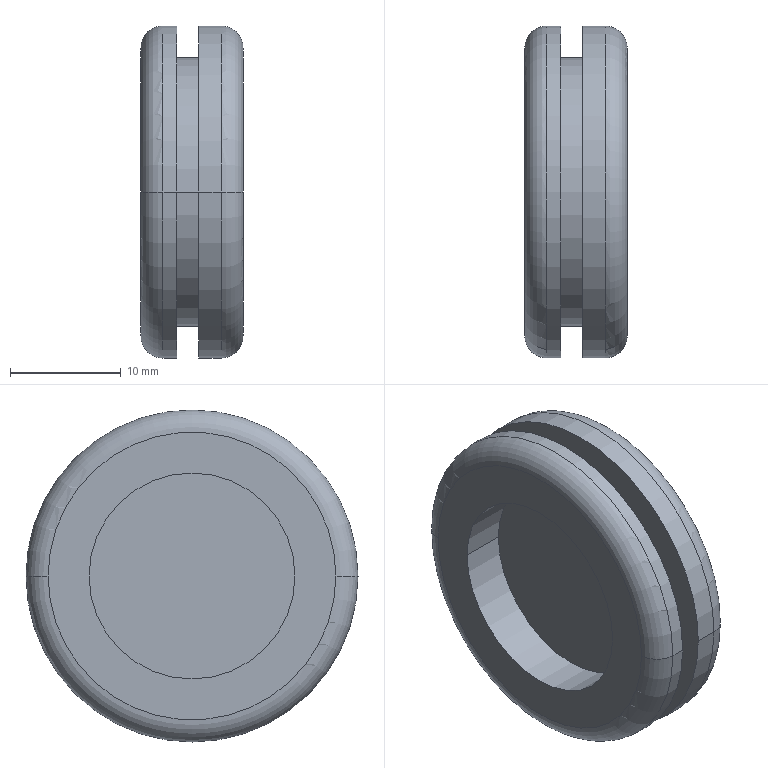Part | STEP file | 60008141 | 1 solid | 20 faces | box 9.25 x 30 x 30 mm | volume 3450 mm3 | cylinder 10 | plane 6 | torus 4 | commonest cylinder face diameters 18.6 x4 30 x4 24.3 x2
STEP:
#1=CARTESIAN_POINT('',(0.,0.,0.));
#2=DIRECTION('',(0.,0.,1.));
#3=DIRECTION('',(1.,0.,0.));
#4=AXIS2_PLACEMENT_3D('',#1,#2,#3);
#5=CARTESIAN_POINT('',(-4.25,9.3,0.));
#6=VERTEX_POINT('',#5);
#7=CARTESIAN_POINT('',(-0.25,9.3,0.));
#8=VERTEX_POINT('',#7);
#9=CARTESIAN_POINT('',(-4.25,9.3,0.));
#10=DIRECTION('',(1.,0.,0.));
#11=VECTOR('',#10,1.);
#12=LINE('',#9,#11);
#13=CARTESIAN_POINT('',(-4.463,0.,0.));
#14=DIRECTION('',(1.,0.,0.));
#15=DIRECTION('',(0.,-1.,0.));
#16=AXIS2_PLACEMENT_3D('',#13,#14,#15);
#17=CYLINDRICAL_SURFACE('',#16,9.3);
#18=CARTESIAN_POINT('',(3.142,0.2125));
#19=DIRECTION('',(0.,1.));
#20=VECTOR('',#19,1.);
#21=LINE('',#18,#20);
#22=(GEOMETRIC_REPRESENTATION_CONTEXT(2)PARAMETRIC_REPRESENTATION_CONTEXT()REPRESENTATION_CONTEXT('',''));
#23=DEFINITIONAL_REPRESENTATION('',(#21),#22);
#24=PCURVE('',#17,#23);
#25=CARTESIAN_POINT('',(-4.463,0.,0.));
#26=DIRECTION('',(1.,0.,0.));
#27=DIRECTION('',(0.,-1.,0.));
#28=AXIS2_PLACEMENT_3D('',#25,#26,#27);
#29=CYLINDRICAL_SURFACE('',#28,9.3);
#30=CARTESIAN_POINT('',(3.142,0.2125));
#31=DIRECTION('',(0.,1.));
#32=VECTOR('',#31,1.);
#33=LINE('',#30,#32);
#34=(GEOMETRIC_REPRESENTATION_CONTEXT(2)PARAMETRIC_REPRESENTATION_CONTEXT()REPRESENTATION_CONTEXT('',''));
#35=DEFINITIONAL_REPRESENTATION('',(#33),#34);
#36=PCURVE('',#29,#35);
#37=SURFACE_CURVE('',#12,(#24,#36),.PCURVE_S1.);
#38=EDGE_CURVE('',#6,#8,#37,.T.);
#39=ORIENTED_EDGE('',*,*,#38,.F.);
#40=CARTESIAN_POINT('',(-4.25,-9.3,0.));
#41=VERTEX_POINT('',#40);
#42=CARTESIAN_POINT('',(-4.25,0.,0.));
#43=DIRECTION('',(1.,0.,0.));
#44=DIRECTION('',(0.,1.,0.));
#45=AXIS2_PLACEMENT_3D('',#42,#43,#44);
#46=CIRCLE('',#45,9.3);
#47=CARTESIAN_POINT('',(3.142,0.2125));
#48=DIRECTION('',(1.,0.));
#49=VECTOR('',#48,1.);
#50=LINE('',#47,#49);
#51=(GEOMETRIC_REPRESENTATION_CONTEXT(2)PARAMETRIC_REPRESENTATION_CONTEXT()REPRESENTATION_CONTEXT('',''));
#52=DEFINITIONAL_REPRESENTATION('',(#50),#51);
#53=PCURVE('',#17,#52);
#54=CARTESIAN_POINT('',(-4.25,0.,0.));
#55=DIRECTION('',(1.,0.,0.));
#56=DIRECTION('',(0.,-1.,0.));
#57=AXIS2_PLACEMENT_3D('',#54,#55,#56);
#58=PLANE('',#57);
#59=CARTESIAN_POINT('',(0.,0.));
#60=DIRECTION('',(-1.,0.));
#61=AXIS2_PLACEMENT_2D('',#59,#60);
#62=CIRCLE('',#61,9.3);
#63=(GEOMETRIC_REPRESENTATION_CONTEXT(2)PARAMETRIC_REPRESENTATION_CONTEXT()REPRESENTATION_CONTEXT('',''));
#64=DEFINITIONAL_REPRESENTATION('',(#62),#63);
#65=PCURVE('',#58,#64);
#66=SURFACE_CURVE('',#46,(#53,#65),.PCURVE_S1.);
#67=EDGE_CURVE('',#6,#41,#66,.T.);
#68=ORIENTED_EDGE('',*,*,#67,.T.);
#69=CARTESIAN_POINT('',(-0.25,-9.3,0.));
#70=VERTEX_POINT('',#69);
#71=CARTESIAN_POINT('',(-4.25,-9.3,0.));
#72=DIRECTION('',(1.,0.,0.));
#73=VECTOR('',#72,1.);
#74=LINE('',#71,#73);
#75=CARTESIAN_POINT('',(6.283,0.2125));
#76=DIRECTION('',(0.,1.));
#77=VECTOR('',#76,1.);
#78=LINE('',#75,#77);
#79=(GEOMETRIC_REPRESENTATION_CONTEXT(2)PARAMETRIC_REPRESENTATION_CONTEXT()REPRESENTATION_CONTEXT('',''));
#80=DEFINITIONAL_REPRESENTATION('',(#78),#79);
#81=PCURVE('',#17,#80);
#82=CARTESIAN_POINT('',(0.,0.2125));
#83=DIRECTION('',(0.,1.));
#84=VECTOR('',#83,1.);
#85=LINE('',#82,#84);
#86=(GEOMETRIC_REPRESENTATION_CONTEXT(2)PARAMETRIC_REPRESENTATION_CONTEXT()REPRESENTATION_CONTEXT('',''));
#87=DEFINITIONAL_REPRESENTATION('',(#85),#86);
#88=PCURVE('',#29,#87);
#89=SURFACE_CURVE('',#74,(#81,#88),.PCURVE_S1.);
#90=EDGE_CURVE('',#41,#70,#89,.T.);
#91=ORIENTED_EDGE('',*,*,#90,.T.);
#92=CARTESIAN_POINT('',(-0.25,0.,0.));
#93=DIRECTION('',(1.,0.,0.));
#94=DIRECTION('',(0.,1.,0.));
#95=AXIS2_PLACEMENT_3D('',#92,#93,#94);
#96=CIRCLE('',#95,9.3);
#97=CARTESIAN_POINT('',(3.142,4.213));
#98=DIRECTION('',(1.,0.));
#99=VECTOR('',#98,1.);
#100=LINE('',#97,#99);
#101=(GEOMETRIC_REPRESENTATION_CONTEXT(2)PARAMETRIC_REPRESENTATION_CONTEXT()REPRESENTATION_CONTEXT('',''));
#102=DEFINITIONAL_REPRESENTATION('',(#100),#101);
#103=PCURVE('',#17,#102);
#104=CARTESIAN_POINT('',(-0.25,0.,0.));
#105=DIRECTION('',(1.,0.,0.));
#106=DIRECTION('',(0.,-1.,0.));
#107=AXIS2_PLACEMENT_3D('',#104,#105,#106);
#108=PLANE('',#107);
#109=CARTESIAN_POINT('',(0.,0.));
#110=DIRECTION('',(-1.,0.));
#111=AXIS2_PLACEMENT_2D('',#109,#110);
#112=CIRCLE('',#111,9.3);
#113=(GEOMETRIC_REPRESENTATION_CONTEXT(2)PARAMETRIC_REPRESENTATION_CONTEXT()REPRESENTATION_CONTEXT('',''));
#114=DEFINITIONAL_REPRESENTATION('',(#112),#113);
#115=PCURVE('',#108,#114);
#116=SURFACE_CURVE('',#96,(#103,#115),.PCURVE_S1.);
#117=EDGE_CURVE('',#8,#70,#116,.T.);
#118=ORIENTED_EDGE('',*,*,#117,.F.);
#119=EDGE_LOOP('',(#39,#68,#91,#118));
#120=FACE_BOUND('',#119,.F.);
#121=ADVANCED_FACE('',(#120),#17,.F.);
#122=ORIENTED_EDGE('',*,*,#38,.T.);
#123=CARTESIAN_POINT('',(-0.25,0.,0.));
#124=DIRECTION('',(-1.,0.,0.));
#125=DIRECTION('',(0.,1.,0.));
#126=AXIS2_PLACEMENT_3D('',#123,#124,#125);
#127=CIRCLE('',#126,9.3);
#128=CARTESIAN_POINT('',(3.142,4.213));
#129=DIRECTION('',(-1.,0.));
#130=VECTOR('',#129,1.);
#131=LINE('',#128,#130);
#132=(GEOMETRIC_REPRESENTATION_CONTEXT(2)PARAMETRIC_REPRESENTATION_CONTEXT()REPRESENTATION_CONTEXT('',''));
#133=DEFINITIONAL_REPRESENTATION('',(#131),#132);
#134=PCURVE('',#29,#133);
#135=CARTESIAN_POINT('',(-9.3,0.));
#136=CARTESIAN_POINT('',(-9.3,16.108));
#137=CARTESIAN_POINT('',(4.65,8.054));
#138=CARTESIAN_POINT('',(18.6,0.));
#139=CARTESIAN_POINT('',(4.65,-8.054));
#140=CARTESIAN_POINT('',(-9.3,-16.108));
#141=CARTESIAN_POINT('',(-9.3,0.));
#142=(BOUNDED_CURVE()B_SPLINE_CURVE(2,(#135,#136,#137,#138,#139,#140,#141),.UNSPECIFIED.,.T.,.F.)B_SPLINE_CURVE_WITH_KNOTS((1,2,2,2,2,1),(-2.094,0.,2.094,4.189,6.283,8.378),.UNSPECIFIED.)CURVE()GEOMETRIC_REPRESENTATION_ITEM()RATIONAL_B_SPLINE_CURVE((1.,0.5,1.,0.5,1.,0.5,1.))REPRESENTATION_ITEM(''));
#143=(GEOMETRIC_REPRESENTATION_CONTEXT(2)PARAMETRIC_REPRESENTATION_CONTEXT()REPRESENTATION_CONTEXT('',''));
#144=DEFINITIONAL_REPRESENTATION('',(#142),#143);
#145=PCURVE('',#108,#144);
#146=SURFACE_CURVE('',#127,(#134,#145),.PCURVE_S1.);
#147=EDGE_CURVE('',#8,#70,#146,.T.);
#148=ORIENTED_EDGE('',*,*,#147,.T.);
#149=ORIENTED_EDGE('',*,*,#90,.F.);
#150=CARTESIAN_POINT('',(-4.25,0.,0.));
#151=DIRECTION('',(-1.,0.,0.));
#152=DIRECTION('',(0.,1.,0.));
#153=AXIS2_PLACEMENT_3D('',#150,#151,#152);
#154=CIRCLE('',#153,9.3);
#155=CARTESIAN_POINT('',(3.142,0.2125));
#156=DIRECTION('',(-1.,0.));
#157=VECTOR('',#156,1.);
#158=LINE('',#155,#157);
#159=(GEOMETRIC_REPRESENTATION_CONTEXT(2)PARAMETRIC_REPRESENTATION_CONTEXT()REPRESENTATION_CONTEXT('',''));
#160=DEFINITIONAL_REPRESENTATION('',(#158),#159);
#161=PCURVE('',#29,#160);
#162=CARTESIAN_POINT('',(-9.3,0.));
#163=CARTESIAN_POINT('',(-9.3,16.108));
#164=CARTESIAN_POINT('',(4.65,8.054));
#165=CARTESIAN_POINT('',(18.6,0.));
#166=CARTESIAN_POINT('',(4.65,-8.054));
#167=CARTESIAN_POINT('',(-9.3,-16.108));
#168=CARTESIAN_POINT('',(-9.3,0.));
#169=(BOUNDED_CURVE()B_SPLINE_CURVE(2,(#162,#163,#164,#165,#166,#167,#168),.UNSPECIFIED.,.T.,.F.)B_SPLINE_CURVE_WITH_KNOTS((1,2,2,2,2,1),(-2.094,0.,2.094,4.189,6.283,8.378),.UNSPECIFIED.)CURVE()GEOMETRIC_REPRESENTATION_ITEM()RATIONAL_B_SPLINE_CURVE((1.,0.5,1.,0.5,1.,0.5,1.))REPRESENTATION_ITEM(''));
#170=(GEOMETRIC_REPRESENTATION_CONTEXT(2)PARAMETRIC_REPRESENTATION_CONTEXT()REPRESENTATION_CONTEXT('',''));
#171=DEFINITIONAL_REPRESENTATION('',(#169),#170);
#172=PCURVE('',#58,#171);
#173=SURFACE_CURVE('',#154,(#161,#172),.PCURVE_S1.);
#174=EDGE_CURVE('',#6,#41,#173,.T.);
#175=ORIENTED_EDGE('',*,*,#174,.F.);
#176=EDGE_LOOP('',(#122,#148,#149,#175));
#177=FACE_BOUND('',#176,.F.);
#178=ADVANCED_FACE('',(#177),#29,.F.);
#179=ORIENTED_EDGE('',*,*,#147,.F.);
#180=ORIENTED_EDGE('',*,*,#117,.T.);
#181=EDGE_LOOP('',(#179,#180));
#182=FACE_BOUND('',#181,.F.);
#183=ADVANCED_FACE('',(#182),#108,.F.);
#184=CARTESIAN_POINT('',(-4.25,13.,0.));
#185=VERTEX_POINT('',#184);
#186=CARTESIAN_POINT('',(-4.25,-13.,0.));
#187=VERTEX_POINT('',#186);
#188=CARTESIAN_POINT('',(-4.25,0.,0.));
#189=DIRECTION('',(1.,0.,0.));
#190=DIRECTION('',(0.,1.,0.));
#191=AXIS2_PLACEMENT_3D('',#188,#189,#190);
#192=CIRCLE('',#191,13.);
#193=CARTESIAN_POINT('',(0.,0.));
#194=DIRECTION('',(-1.,0.));
#195=AXIS2_PLACEMENT_2D('',#193,#194);
#196=CIRCLE('',#195,13.);
#197=(GEOMETRIC_REPRESENTATION_CONTEXT(2)PARAMETRIC_REPRESENTATION_CONTEXT()REPRESENTATION_CONTEXT('',''));
#198=DEFINITIONAL_REPRESENTATION('',(#196),#197);
#199=PCURVE('',#58,#198);
#200=CARTESIAN_POINT('',(-2.25,0.,0.));
#201=DIRECTION('',(1.,0.,0.));
#202=DIRECTION('',(0.,-1.,0.));
#203=AXIS2_PLACEMENT_3D('',#200,#201,#202);
#204=TOROIDAL_SURFACE('',#203,13.,2.);
#205=CARTESIAN_POINT('',(3.142,4.712));
#206=DIRECTION('',(1.,0.));
#207=VECTOR('',#206,1.);
#208=LINE('',#205,#207);
#209=(GEOMETRIC_REPRESENTATION_CONTEXT(2)PARAMETRIC_REPRESENTATION_CONTEXT()REPRESENTATION_CONTEXT('',''));
#210=DEFINITIONAL_REPRESENTATION('',(#208),#209);
#211=PCURVE('',#204,#210);
#212=SURFACE_CURVE('',#192,(#199,#211),.PCURVE_S1.);
#213=EDGE_CURVE('',#185,#187,#212,.T.);
#214=ORIENTED_EDGE('',*,*,#213,.T.);
#215=CARTESIAN_POINT('',(-4.25,0.,0.));
#216=DIRECTION('',(-1.,0.,0.));
#217=DIRECTION('',(0.,1.,0.));
#218=AXIS2_PLACEMENT_3D('',#215,#216,#217);
#219=CIRCLE('',#218,13.);
#220=CARTESIAN_POINT('',(-13.,0.));
#221=CARTESIAN_POINT('',(-13.,22.517));
#222=CARTESIAN_POINT('',(6.5,11.258));
#223=CARTESIAN_POINT('',(26.,0.));
#224=CARTESIAN_POINT('',(6.5,-11.258));
#225=CARTESIAN_POINT('',(-13.,-22.517));
#226=CARTESIAN_POINT('',(-13.,0.));
#227=(BOUNDED_CURVE()B_SPLINE_CURVE(2,(#220,#221,#222,#223,#224,#225,#226),.UNSPECIFIED.,.T.,.F.)B_SPLINE_CURVE_WITH_KNOTS((1,2,2,2,2,1),(-2.094,0.,2.094,4.189,6.283,8.378),.UNSPECIFIED.)CURVE()GEOMETRIC_REPRESENTATION_ITEM()RATIONAL_B_SPLINE_CURVE((1.,0.5,1.,0.5,1.,0.5,1.))REPRESENTATION_ITEM(''));
#228=(GEOMETRIC_REPRESENTATION_CONTEXT(2)PARAMETRIC_REPRESENTATION_CONTEXT()REPRESENTATION_CONTEXT('',''));
#229=DEFINITIONAL_REPRESENTATION('',(#227),#228);
#230=PCURVE('',#58,#229);
#231=CARTESIAN_POINT('',(-2.25,0.,0.));
#232=DIRECTION('',(1.,0.,0.));
#233=DIRECTION('',(0.,-1.,0.));
#234=AXIS2_PLACEMENT_3D('',#231,#232,#233);
#235=TOROIDAL_SURFACE('',#234,13.,2.);
#236=CARTESIAN_POINT('',(3.142,4.712));
#237=DIRECTION('',(-1.,0.));
#238=VECTOR('',#237,1.);
#239=LINE('',#236,#238);
#240=(GEOMETRIC_REPRESENTATION_CONTEXT(2)PARAMETRIC_REPRESENTATION_CONTEXT()REPRESENTATION_CONTEXT('',''));
#241=DEFINITIONAL_REPRESENTATION('',(#239),#240);
#242=PCURVE('',#235,#241);
#243=SURFACE_CURVE('',#219,(#230,#242),.PCURVE_S1.);
#244=EDGE_CURVE('',#185,#187,#243,.T.);
#245=ORIENTED_EDGE('',*,*,#244,.F.);
#246=EDGE_LOOP('',(#214,#245));
#247=FACE_BOUND('',#246,.F.);
#248=ORIENTED_EDGE('',*,*,#174,.T.);
#249=ORIENTED_EDGE('',*,*,#67,.F.);
#250=EDGE_LOOP('',(#248,#249));
#251=FACE_BOUND('',#250,.F.);
#252=ADVANCED_FACE('',(#247,#251),#58,.F.);
#253=ORIENTED_EDGE('',*,*,#213,.T.);
#254=CARTESIAN_POINT('',(-2.25,-15.,0.));
#255=VERTEX_POINT('',#254);
#256=CARTESIAN_POINT('',(-2.25,-13.,0.));
#257=DIRECTION('',(0.,0.,-1.));
#258=DIRECTION('',(0.,-1.,0.));
#259=AXIS2_PLACEMENT_3D('',#256,#257,#258);
#260=CIRCLE('',#259,2.);
#261=CARTESIAN_POINT('',(6.283,6.283));
#262=DIRECTION('',(0.,-1.));
#263=VECTOR('',#262,1.);
#264=LINE('',#261,#263);
#265=(GEOMETRIC_REPRESENTATION_CONTEXT(2)PARAMETRIC_REPRESENTATION_CONTEXT()REPRESENTATION_CONTEXT('',''));
#266=DEFINITIONAL_REPRESENTATION('',(#264),#265);
#267=PCURVE('',#204,#266);
#268=CARTESIAN_POINT('',(0.,6.283));
#269=DIRECTION('',(0.,-1.));
#270=VECTOR('',#269,1.);
#271=LINE('',#268,#270);
#272=(GEOMETRIC_REPRESENTATION_CONTEXT(2)PARAMETRIC_REPRESENTATION_CONTEXT()REPRESENTATION_CONTEXT('',''));
#273=DEFINITIONAL_REPRESENTATION('',(#271),#272);
#274=PCURVE('',#235,#273);
#275=SURFACE_CURVE('',#260,(#267,#274),.PCURVE_S1.);
#276=EDGE_CURVE('',#255,#187,#275,.T.);
#277=ORIENTED_EDGE('',*,*,#276,.F.);
#278=CARTESIAN_POINT('',(-2.25,15.,0.));
#279=VERTEX_POINT('',#278);
#280=CARTESIAN_POINT('',(-2.25,0.,0.));
#281=DIRECTION('',(1.,0.,0.));
#282=DIRECTION('',(0.,1.,0.));
#283=AXIS2_PLACEMENT_3D('',#280,#281,#282);
#284=CIRCLE('',#283,15.);
#285=CARTESIAN_POINT('',(3.142,6.283));
#286=DIRECTION('',(1.,0.));
#287=VECTOR('',#286,1.);
#288=LINE('',#285,#287);
#289=(GEOMETRIC_REPRESENTATION_CONTEXT(2)PARAMETRIC_REPRESENTATION_CONTEXT()REPRESENTATION_CONTEXT('',''));
#290=DEFINITIONAL_REPRESENTATION('',(#288),#289);
#291=PCURVE('',#204,#290);
#292=CARTESIAN_POINT('',(-4.463,0.,0.));
#293=DIRECTION('',(1.,0.,0.));
#294=DIRECTION('',(0.,-1.,0.));
#295=AXIS2_PLACEMENT_3D('',#292,#293,#294);
#296=CYLINDRICAL_SURFACE('',#295,15.);
#297=CARTESIAN_POINT('',(3.142,2.212));
#298=DIRECTION('',(1.,0.));
#299=VECTOR('',#298,1.);
#300=LINE('',#297,#299);
#301=(GEOMETRIC_REPRESENTATION_CONTEXT(2)PARAMETRIC_REPRESENTATION_CONTEXT()REPRESENTATION_CONTEXT('',''));
#302=DEFINITIONAL_REPRESENTATION('',(#300),#301);
#303=PCURVE('',#296,#302);
#304=SURFACE_CURVE('',#284,(#291,#303),.PCURVE_S1.);
#305=EDGE_CURVE('',#279,#255,#304,.T.);
#306=ORIENTED_EDGE('',*,*,#305,.F.);
#307=CARTESIAN_POINT('',(-2.25,13.,0.));
#308=DIRECTION('',(0.,0.,1.));
#309=DIRECTION('',(0.,1.,0.));
#310=AXIS2_PLACEMENT_3D('',#307,#308,#309);
#311=CIRCLE('',#310,2.);
#312=CARTESIAN_POINT('',(3.142,6.283));
#313=DIRECTION('',(0.,-1.));
#314=VECTOR('',#313,1.);
#315=LINE('',#312,#314);
#316=(GEOMETRIC_REPRESENTATION_CONTEXT(2)PARAMETRIC_REPRESENTATION_CONTEXT()REPRESENTATION_CONTEXT('',''));
#317=DEFINITIONAL_REPRESENTATION('',(#315),#316);
#318=PCURVE('',#204,#317);
#319=CARTESIAN_POINT('',(3.142,6.283));
#320=DIRECTION('',(0.,-1.));
#321=VECTOR('',#320,1.);
#322=LINE('',#319,#321);
#323=(GEOMETRIC_REPRESENTATION_CONTEXT(2)PARAMETRIC_REPRESENTATION_CONTEXT()REPRESENTATION_CONTEXT('',''));
#324=DEFINITIONAL_REPRESENTATION('',(#322),#323);
#325=PCURVE('',#235,#324);
#326=SURFACE_CURVE('',#311,(#318,#325),.PCURVE_S1.);
#327=EDGE_CURVE('',#279,#185,#326,.T.);
#328=ORIENTED_EDGE('',*,*,#327,.T.);
#329=EDGE_LOOP('',(#253,#277,#306,#328));
#330=FACE_BOUND('',#329,.T.);
#331=ADVANCED_FACE('',(#330),#204,.T.);
#332=CARTESIAN_POINT('',(-2.25,0.,0.));
#333=DIRECTION('',(-1.,0.,0.));
#334=DIRECTION('',(0.,1.,0.));
#335=AXIS2_PLACEMENT_3D('',#332,#333,#334);
#336=CIRCLE('',#335,15.);
#337=CARTESIAN_POINT('',(3.142,6.283));
#338=DIRECTION('',(-1.,0.));
#339=VECTOR('',#338,1.);
#340=LINE('',#337,#339);
#341=(GEOMETRIC_REPRESENTATION_CONTEXT(2)PARAMETRIC_REPRESENTATION_CONTEXT()REPRESENTATION_CONTEXT('',''));
#342=DEFINITIONAL_REPRESENTATION('',(#340),#341);
#343=PCURVE('',#235,#342);
#344=CARTESIAN_POINT('',(-4.463,0.,0.));
#345=DIRECTION('',(1.,0.,0.));
#346=DIRECTION('',(0.,-1.,0.));
#347=AXIS2_PLACEMENT_3D('',#344,#345,#346);
#348=CYLINDRICAL_SURFACE('',#347,15.);
#349=CARTESIAN_POINT('',(3.142,2.212));
#350=DIRECTION('',(-1.,0.));
#351=VECTOR('',#350,1.);
#352=LINE('',#349,#351);
#353=(GEOMETRIC_REPRESENTATION_CONTEXT(2)PARAMETRIC_REPRESENTATION_CONTEXT()REPRESENTATION_CONTEXT('',''));
#354=DEFINITIONAL_REPRESENTATION('',(#352),#353);
#355=PCURVE('',#348,#354);
#356=SURFACE_CURVE('',#336,(#343,#355),.PCURVE_S1.);
#357=EDGE_CURVE('',#279,#255,#356,.T.);
#358=ORIENTED_EDGE('',*,*,#357,.T.);
#359=ORIENTED_EDGE('',*,*,#276,.T.);
#360=ORIENTED_EDGE('',*,*,#244,.F.);
#361=ORIENTED_EDGE('',*,*,#327,.F.);
#362=EDGE_LOOP('',(#358,#359,#360,#361));
#363=FACE_BOUND('',#362,.T.);
#364=ADVANCED_FACE('',(#363),#235,.T.);
#365=CARTESIAN_POINT('',(-1.,15.,0.));
#366=VERTEX_POINT('',#365);
#367=CARTESIAN_POINT('',(-1.,-15.,0.));
#368=VERTEX_POINT('',#367);
#369=CARTESIAN_POINT('',(-1.,0.,0.));
#370=DIRECTION('',(-1.,0.,0.));
#371=DIRECTION('',(0.,1.,0.));
#372=AXIS2_PLACEMENT_3D('',#369,#370,#371);
#373=CIRCLE('',#372,15.);
#374=CARTESIAN_POINT('',(3.142,3.462));
#375=DIRECTION('',(-1.,0.));
#376=VECTOR('',#375,1.);
#377=LINE('',#374,#376);
#378=(GEOMETRIC_REPRESENTATION_CONTEXT(2)PARAMETRIC_REPRESENTATION_CONTEXT()REPRESENTATION_CONTEXT('',''));
#379=DEFINITIONAL_REPRESENTATION('',(#377),#378);
#380=PCURVE('',#348,#379);
#381=CARTESIAN_POINT('',(-1.,0.,0.));
#382=DIRECTION('',(1.,0.,0.));
#383=DIRECTION('',(0.,-1.,0.));
#384=AXIS2_PLACEMENT_3D('',#381,#382,#383);
#385=PLANE('',#384);
#386=CARTESIAN_POINT('',(-15.,0.));
#387=CARTESIAN_POINT('',(-15.,25.981));
#388=CARTESIAN_POINT('',(7.5,12.99));
#389=CARTESIAN_POINT('',(30.,0.));
#390=CARTESIAN_POINT('',(7.5,-12.99));
#391=CARTESIAN_POINT('',(-15.,-25.981));
#392=CARTESIAN_POINT('',(-15.,0.));
#393=(BOUNDED_CURVE()B_SPLINE_CURVE(2,(#386,#387,#388,#389,#390,#391,#392),.UNSPECIFIED.,.T.,.F.)B_SPLINE_CURVE_WITH_KNOTS((1,2,2,2,2,1),(-2.094,0.,2.094,4.189,6.283,8.378),.UNSPECIFIED.)CURVE()GEOMETRIC_REPRESENTATION_ITEM()RATIONAL_B_SPLINE_CURVE((1.,0.5,1.,0.5,1.,0.5,1.))REPRESENTATION_ITEM(''));
#394=(GEOMETRIC_REPRESENTATION_CONTEXT(2)PARAMETRIC_REPRESENTATION_CONTEXT()REPRESENTATION_CONTEXT('',''));
#395=DEFINITIONAL_REPRESENTATION('',(#393),#394);
#396=PCURVE('',#385,#395);
#397=SURFACE_CURVE('',#373,(#380,#396),.PCURVE_S1.);
#398=EDGE_CURVE('',#366,#368,#397,.T.);
#399=ORIENTED_EDGE('',*,*,#398,.T.);
#400=CARTESIAN_POINT('',(-1.,-15.,0.));
#401=DIRECTION('',(-1.,0.,0.));
#402=VECTOR('',#401,1.);
#403=LINE('',#400,#402);
#404=CARTESIAN_POINT('',(0.,3.462));
#405=DIRECTION('',(0.,-1.));
#406=VECTOR('',#405,1.);
#407=LINE('',#404,#406);
#408=(GEOMETRIC_REPRESENTATION_CONTEXT(2)PARAMETRIC_REPRESENTATION_CONTEXT()REPRESENTATION_CONTEXT('',''));
#409=DEFINITIONAL_REPRESENTATION('',(#407),#408);
#410=PCURVE('',#348,#409);
#411=CARTESIAN_POINT('',(6.283,3.462));
#412=DIRECTION('',(0.,-1.));
#413=VECTOR('',#412,1.);
#414=LINE('',#411,#413);
#415=(GEOMETRIC_REPRESENTATION_CONTEXT(2)PARAMETRIC_REPRESENTATION_CONTEXT()REPRESENTATION_CONTEXT('',''));
#416=DEFINITIONAL_REPRESENTATION('',(#414),#415);
#417=PCURVE('',#296,#416);
#418=SURFACE_CURVE('',#403,(#410,#417),.PCURVE_S1.);
#419=EDGE_CURVE('',#368,#255,#418,.T.);
#420=ORIENTED_EDGE('',*,*,#419,.T.);
#421=ORIENTED_EDGE('',*,*,#357,.F.);
#422=CARTESIAN_POINT('',(-1.,15.,0.));
#423=DIRECTION('',(-1.,0.,0.));
#424=VECTOR('',#423,1.);
#425=LINE('',#422,#424);
#426=CARTESIAN_POINT('',(3.142,3.462));
#427=DIRECTION('',(0.,-1.));
#428=VECTOR('',#427,1.);
#429=LINE('',#426,#428);
#430=(GEOMETRIC_REPRESENTATION_CONTEXT(2)PARAMETRIC_REPRESENTATION_CONTEXT()REPRESENTATION_CONTEXT('',''));
#431=DEFINITIONAL_REPRESENTATION('',(#429),#430);
#432=PCURVE('',#348,#431);
#433=CARTESIAN_POINT('',(3.142,3.462));
#434=DIRECTION('',(0.,-1.));
#435=VECTOR('',#434,1.);
#436=LINE('',#433,#435);
#437=(GEOMETRIC_REPRESENTATION_CONTEXT(2)PARAMETRIC_REPRESENTATION_CONTEXT()REPRESENTATION_CONTEXT('',''));
#438=DEFINITIONAL_REPRESENTATION('',(#436),#437);
#439=PCURVE('',#296,#438);
#440=SURFACE_CURVE('',#425,(#432,#439),.PCURVE_S1.);
#441=EDGE_CURVE('',#366,#279,#440,.T.);
#442=ORIENTED_EDGE('',*,*,#441,.F.);
#443=EDGE_LOOP('',(#399,#420,#421,#442));
#444=FACE_BOUND('',#443,.T.);
#445=ADVANCED_FACE('',(#444),#348,.T.);
#446=ORIENTED_EDGE('',*,*,#305,.T.);
#447=ORIENTED_EDGE('',*,*,#419,.F.);
#448=CARTESIAN_POINT('',(-1.,0.,0.));
#449=DIRECTION('',(1.,0.,0.));
#450=DIRECTION('',(0.,1.,0.));
#451=AXIS2_PLACEMENT_3D('',#448,#449,#450);
#452=CIRCLE('',#451,15.);
#453=CARTESIAN_POINT('',(3.142,3.462));
#454=DIRECTION('',(1.,0.));
#455=VECTOR('',#454,1.);
#456=LINE('',#453,#455);
#457=(GEOMETRIC_REPRESENTATION_CONTEXT(2)PARAMETRIC_REPRESENTATION_CONTEXT()REPRESENTATION_CONTEXT('',''));
#458=DEFINITIONAL_REPRESENTATION('',(#456),#457);
#459=PCURVE('',#296,#458);
#460=CARTESIAN_POINT('',(0.,0.));
#461=DIRECTION('',(-1.,0.));
#462=AXIS2_PLACEMENT_2D('',#460,#461);
#463=CIRCLE('',#462,15.);
#464=(GEOMETRIC_REPRESENTATION_CONTEXT(2)PARAMETRIC_REPRESENTATION_CONTEXT()REPRESENTATION_CONTEXT('',''));
#465=DEFINITIONAL_REPRESENTATION('',(#463),#464);
#466=PCURVE('',#385,#465);
#467=SURFACE_CURVE('',#452,(#459,#466),.PCURVE_S1.);
#468=EDGE_CURVE('',#366,#368,#467,.T.);
#469=ORIENTED_EDGE('',*,*,#468,.F.);
#470=ORIENTED_EDGE('',*,*,#441,.T.);
#471=EDGE_LOOP('',(#446,#447,#469,#470));
#472=FACE_BOUND('',#471,.T.);
#473=ADVANCED_FACE('',(#472),#296,.T.);
#474=ORIENTED_EDGE('',*,*,#398,.T.);
#475=ORIENTED_EDGE('',*,*,#468,.F.);
#476=EDGE_LOOP('',(#474,#475));
#477=FACE_BOUND('',#476,.F.);
#478=CARTESIAN_POINT('',(-1.,12.15,0.));
#479=VERTEX_POINT('',#478);
#480=CARTESIAN_POINT('',(-1.,-12.15,0.));
#481=VERTEX_POINT('',#480);
#482=CARTESIAN_POINT('',(-1.,0.,0.));
#483=DIRECTION('',(1.,0.,0.));
#484=DIRECTION('',(0.,1.,0.));
#485=AXIS2_PLACEMENT_3D('',#482,#483,#484);
#486=CIRCLE('',#485,12.15);
#487=CARTESIAN_POINT('',(0.,0.));
#488=DIRECTION('',(-1.,0.));
#489=AXIS2_PLACEMENT_2D('',#487,#488);
#490=CIRCLE('',#489,12.15);
#491=(GEOMETRIC_REPRESENTATION_CONTEXT(2)PARAMETRIC_REPRESENTATION_CONTEXT()REPRESENTATION_CONTEXT('',''));
#492=DEFINITIONAL_REPRESENTATION('',(#490),#491);
#493=PCURVE('',#385,#492);
#494=CARTESIAN_POINT('',(-4.463,0.,0.));
#495=DIRECTION('',(1.,0.,0.));
#496=DIRECTION('',(0.,-1.,0.));
#497=AXIS2_PLACEMENT_3D('',#494,#495,#496);
#498=CYLINDRICAL_SURFACE('',#497,12.15);
#499=CARTESIAN_POINT('',(3.142,3.462));
#500=DIRECTION('',(1.,0.));
#501=VECTOR('',#500,1.);
#502=LINE('',#499,#501);
#503=(GEOMETRIC_REPRESENTATION_CONTEXT(2)PARAMETRIC_REPRESENTATION_CONTEXT()REPRESENTATION_CONTEXT('',''));
#504=DEFINITIONAL_REPRESENTATION('',(#502),#503);
#505=PCURVE('',#498,#504);
#506=SURFACE_CURVE('',#486,(#493,#505),.PCURVE_S1.);
#507=EDGE_CURVE('',#479,#481,#506,.T.);
#508=ORIENTED_EDGE('',*,*,#507,.T.);
#509=CARTESIAN_POINT('',(-1.,0.,0.));
#510=DIRECTION('',(-1.,0.,0.));
#511=DIRECTION('',(0.,1.,0.));
#512=AXIS2_PLACEMENT_3D('',#509,#510,#511);
#513=CIRCLE('',#512,12.15);
#514=CARTESIAN_POINT('',(-12.15,0.));
#515=CARTESIAN_POINT('',(-12.15,21.044));
#516=CARTESIAN_POINT('',(6.075,10.522));
#517=CARTESIAN_POINT('',(24.3,0.));
#518=CARTESIAN_POINT('',(6.075,-10.522));
#519=CARTESIAN_POINT('',(-12.15,-21.044));
#520=CARTESIAN_POINT('',(-12.15,0.));
#521=(BOUNDED_CURVE()B_SPLINE_CURVE(2,(#514,#515,#516,#517,#518,#519,#520),.UNSPECIFIED.,.T.,.F.)B_SPLINE_CURVE_WITH_KNOTS((1,2,2,2,2,1),(-2.094,0.,2.094,4.189,6.283,8.378),.UNSPECIFIED.)CURVE()GEOMETRIC_REPRESENTATION_ITEM()RATIONAL_B_SPLINE_CURVE((1.,0.5,1.,0.5,1.,0.5,1.))REPRESENTATION_ITEM(''));
#522=(GEOMETRIC_REPRESENTATION_CONTEXT(2)PARAMETRIC_REPRESENTATION_CONTEXT()REPRESENTATION_CONTEXT('',''));
#523=DEFINITIONAL_REPRESENTATION('',(#521),#522);
#524=PCURVE('',#385,#523);
#525=CARTESIAN_POINT('',(-4.463,0.,0.));
#526=DIRECTION('',(1.,0.,0.));
#527=DIRECTION('',(0.,-1.,0.));
#528=AXIS2_PLACEMENT_3D('',#525,#526,#527);
#529=CYLINDRICAL_SURFACE('',#528,12.15);
#530=CARTESIAN_POINT('',(3.142,3.462));
#531=DIRECTION('',(-1.,0.));
#532=VECTOR('',#531,1.);
#533=LINE('',#530,#532);
#534=(GEOMETRIC_REPRESENTATION_CONTEXT(2)PARAMETRIC_REPRESENTATION_CONTEXT()REPRESENTATION_CONTEXT('',''));
#535=DEFINITIONAL_REPRESENTATION('',(#533),#534);
#536=PCURVE('',#529,#535);
#537=SURFACE_CURVE('',#513,(#524,#536),.PCURVE_S1.);
#538=EDGE_CURVE('',#479,#481,#537,.T.);
#539=ORIENTED_EDGE('',*,*,#538,.F.);
#540=EDGE_LOOP('',(#508,#539));
#541=FACE_BOUND('',#540,.F.);
#542=ADVANCED_FACE('',(#477,#541),#385,.T.);
#543=ORIENTED_EDGE('',*,*,#507,.T.);
#544=CARTESIAN_POINT('',(1.,-12.15,0.));
#545=VERTEX_POINT('',#544);
#546=CARTESIAN_POINT('',(-1.,-12.15,0.));
#547=DIRECTION('',(1.,0.,0.));
#548=VECTOR('',#547,1.);
#549=LINE('',#546,#548);
#550=CARTESIAN_POINT('',(6.283,3.462));
#551=DIRECTION('',(0.,1.));
#552=VECTOR('',#551,1.);
#553=LINE('',#550,#552);
#554=(GEOMETRIC_REPRESENTATION_CONTEXT(2)PARAMETRIC_REPRESENTATION_CONTEXT()REPRESENTATION_CONTEXT('',''));
#555=DEFINITIONAL_REPRESENTATION('',(#553),#554);
#556=PCURVE('',#498,#555);
#557=CARTESIAN_POINT('',(0.,3.462));
#558=DIRECTION('',(0.,1.));
#559=VECTOR('',#558,1.);
#560=LINE('',#557,#559);
#561=(GEOMETRIC_REPRESENTATION_CONTEXT(2)PARAMETRIC_REPRESENTATION_CONTEXT()REPRESENTATION_CONTEXT('',''));
#562=DEFINITIONAL_REPRESENTATION('',(#560),#561);
#563=PCURVE('',#529,#562);
#564=SURFACE_CURVE('',#549,(#556,#563),.PCURVE_S1.);
#565=EDGE_CURVE('',#481,#545,#564,.T.);
#566=ORIENTED_EDGE('',*,*,#565,.T.);
#567=CARTESIAN_POINT('',(1.,12.15,0.));
#568=VERTEX_POINT('',#567);
#569=CARTESIAN_POINT('',(1.,0.,0.));
#570=DIRECTION('',(1.,0.,0.));
#571=DIRECTION('',(0.,1.,0.));
#572=AXIS2_PLACEMENT_3D('',#569,#570,#571);
#573=CIRCLE('',#572,12.15);
#574=CARTESIAN_POINT('',(3.142,5.463));
#575=DIRECTION('',(1.,0.));
#576=VECTOR('',#575,1.);
#577=LINE('',#574,#576);
#578=(GEOMETRIC_REPRESENTATION_CONTEXT(2)PARAMETRIC_REPRESENTATION_CONTEXT()REPRESENTATION_CONTEXT('',''));
#579=DEFINITIONAL_REPRESENTATION('',(#577),#578);
#580=PCURVE('',#498,#579);
#581=CARTESIAN_POINT('',(1.,0.,0.));
#582=DIRECTION('',(1.,0.,0.));
#583=DIRECTION('',(0.,-1.,0.));
#584=AXIS2_PLACEMENT_3D('',#581,#582,#583);
#585=PLANE('',#584);
#586=CARTESIAN_POINT('',(0.,0.));
#587=DIRECTION('',(-1.,0.));
#588=AXIS2_PLACEMENT_2D('',#586,#587);
#589=CIRCLE('',#588,12.15);
#590=(GEOMETRIC_REPRESENTATION_CONTEXT(2)PARAMETRIC_REPRESENTATION_CONTEXT()REPRESENTATION_CONTEXT('',''));
#591=DEFINITIONAL_REPRESENTATION('',(#589),#590);
#592=PCURVE('',#585,#591);
#593=SURFACE_CURVE('',#573,(#580,#592),.PCURVE_S1.);
#594=EDGE_CURVE('',#568,#545,#593,.T.);
#595=ORIENTED_EDGE('',*,*,#594,.F.);
#596=CARTESIAN_POINT('',(1.,12.15,0.));
#597=DIRECTION('',(-1.,0.,0.));
#598=VECTOR('',#597,1.);
#599=LINE('',#596,#598);
#600=CARTESIAN_POINT('',(3.142,5.463));
#601=DIRECTION('',(0.,-1.));
#602=VECTOR('',#601,1.);
#603=LINE('',#600,#602);
#604=(GEOMETRIC_REPRESENTATION_CONTEXT(2)PARAMETRIC_REPRESENTATION_CONTEXT()REPRESENTATION_CONTEXT('',''));
#605=DEFINITIONAL_REPRESENTATION('',(#603),#604);
#606=PCURVE('',#498,#605);
#607=CARTESIAN_POINT('',(3.142,5.463));
#608=DIRECTION('',(0.,-1.));
#609=VECTOR('',#608,1.);
#610=LINE('',#607,#609);
#611=(GEOMETRIC_REPRESENTATION_CONTEXT(2)PARAMETRIC_REPRESENTATION_CONTEXT()REPRESENTATION_CONTEXT('',''));
#612=DEFINITIONAL_REPRESENTATION('',(#610),#611);
#613=PCURVE('',#529,#612);
#614=SURFACE_CURVE('',#599,(#606,#613),.PCURVE_S1.);
#615=EDGE_CURVE('',#568,#479,#614,.T.);
#616=ORIENTED_EDGE('',*,*,#615,.T.);
#617=EDGE_LOOP('',(#543,#566,#595,#616));
#618=FACE_BOUND('',#617,.T.);
#619=ADVANCED_FACE('',(#618),#498,.T.);
#620=ORIENTED_EDGE('',*,*,#538,.F.);
#621=ORIENTED_EDGE('',*,*,#615,.F.);
#622=CARTESIAN_POINT('',(1.,0.,0.));
#623=DIRECTION('',(-1.,0.,0.));
#624=DIRECTION('',(0.,1.,0.));
#625=AXIS2_PLACEMENT_3D('',#622,#623,#624);
#626=CIRCLE('',#625,12.15);
#627=CARTESIAN_POINT('',(3.142,5.463));
#628=DIRECTION('',(-1.,0.));
#629=VECTOR('',#628,1.);
#630=LINE('',#627,#629);
#631=(GEOMETRIC_REPRESENTATION_CONTEXT(2)PARAMETRIC_REPRESENTATION_CONTEXT()REPRESENTATION_CONTEXT('',''));
#632=DEFINITIONAL_REPRESENTATION('',(#630),#631);
#633=PCURVE('',#529,#632);
#634=CARTESIAN_POINT('',(-12.15,0.));
#635=CARTESIAN_POINT('',(-12.15,21.044));
#636=CARTESIAN_POINT('',(6.075,10.522));
#637=CARTESIAN_POINT('',(24.3,0.));
#638=CARTESIAN_POINT('',(6.075,-10.522));
#639=CARTESIAN_POINT('',(-12.15,-21.044));
#640=CARTESIAN_POINT('',(-12.15,0.));
#641=(BOUNDED_CURVE()B_SPLINE_CURVE(2,(#634,#635,#636,#637,#638,#639,#640),.UNSPECIFIED.,.T.,.F.)B_SPLINE_CURVE_WITH_KNOTS((1,2,2,2,2,1),(-2.094,0.,2.094,4.189,6.283,8.378),.UNSPECIFIED.)CURVE()GEOMETRIC_REPRESENTATION_ITEM()RATIONAL_B_SPLINE_CURVE((1.,0.5,1.,0.5,1.,0.5,1.))REPRESENTATION_ITEM(''));
#642=(GEOMETRIC_REPRESENTATION_CONTEXT(2)PARAMETRIC_REPRESENTATION_CONTEXT()REPRESENTATION_CONTEXT('',''));
#643=DEFINITIONAL_REPRESENTATION('',(#641),#642);
#644=PCURVE('',#585,#643);
#645=SURFACE_CURVE('',#626,(#633,#644),.PCURVE_S1.);
#646=EDGE_CURVE('',#568,#545,#645,.T.);
#647=ORIENTED_EDGE('',*,*,#646,.T.);
#648=ORIENTED_EDGE('',*,*,#565,.F.);
#649=EDGE_LOOP('',(#620,#621,#647,#648));
#650=FACE_BOUND('',#649,.T.);
#651=ADVANCED_FACE('',(#650),#529,.T.);
#652=CARTESIAN_POINT('',(1.,15.,0.));
#653=VERTEX_POINT('',#652);
#654=CARTESIAN_POINT('',(1.,-15.,0.));
#655=VERTEX_POINT('',#654);
#656=CARTESIAN_POINT('',(1.,0.,0.));
#657=DIRECTION('',(1.,0.,0.));
#658=DIRECTION('',(0.,1.,0.));
#659=AXIS2_PLACEMENT_3D('',#656,#657,#658);
#660=CIRCLE('',#659,15.);
#661=CARTESIAN_POINT('',(0.,0.));
#662=DIRECTION('',(-1.,0.));
#663=AXIS2_PLACEMENT_2D('',#661,#662);
#664=CIRCLE('',#663,15.);
#665=(GEOMETRIC_REPRESENTATION_CONTEXT(2)PARAMETRIC_REPRESENTATION_CONTEXT()REPRESENTATION_CONTEXT('',''));
#666=DEFINITIONAL_REPRESENTATION('',(#664),#665);
#667=PCURVE('',#585,#666);
#668=CARTESIAN_POINT('',(5.25,0.,0.));
#669=DIRECTION('',(1.,0.,0.));
#670=DIRECTION('',(0.,-1.,0.));
#671=AXIS2_PLACEMENT_3D('',#668,#669,#670);
#672=CYLINDRICAL_SURFACE('',#671,15.);
#673=CARTESIAN_POINT('',(3.142,-4.25));
#674=DIRECTION('',(1.,0.));
#675=VECTOR('',#674,1.);
#676=LINE('',#673,#675);
#677=(GEOMETRIC_REPRESENTATION_CONTEXT(2)PARAMETRIC_REPRESENTATION_CONTEXT()REPRESENTATION_CONTEXT('',''));
#678=DEFINITIONAL_REPRESENTATION('',(#676),#677);
#679=PCURVE('',#672,#678);
#680=SURFACE_CURVE('',#660,(#667,#679),.PCURVE_S1.);
#681=EDGE_CURVE('',#653,#655,#680,.T.);
#682=ORIENTED_EDGE('',*,*,#681,.T.);
#683=CARTESIAN_POINT('',(1.,0.,0.));
#684=DIRECTION('',(-1.,0.,0.));
#685=DIRECTION('',(0.,1.,0.));
#686=AXIS2_PLACEMENT_3D('',#683,#684,#685);
#687=CIRCLE('',#686,15.);
#688=CARTESIAN_POINT('',(-15.,0.));
#689=CARTESIAN_POINT('',(-15.,25.981));
#690=CARTESIAN_POINT('',(7.5,12.99));
#691=CARTESIAN_POINT('',(30.,0.));
#692=CARTESIAN_POINT('',(7.5,-12.99));
#693=CARTESIAN_POINT('',(-15.,-25.981));
#694=CARTESIAN_POINT('',(-15.,0.));
#695=(BOUNDED_CURVE()B_SPLINE_CURVE(2,(#688,#689,#690,#691,#692,#693,#694),.UNSPECIFIED.,.T.,.F.)B_SPLINE_CURVE_WITH_KNOTS((1,2,2,2,2,1),(-2.094,0.,2.094,4.189,6.283,8.378),.UNSPECIFIED.)CURVE()GEOMETRIC_REPRESENTATION_ITEM()RATIONAL_B_SPLINE_CURVE((1.,0.5,1.,0.5,1.,0.5,1.))REPRESENTATION_ITEM(''));
#696=(GEOMETRIC_REPRESENTATION_CONTEXT(2)PARAMETRIC_REPRESENTATION_CONTEXT()REPRESENTATION_CONTEXT('',''));
#697=DEFINITIONAL_REPRESENTATION('',(#695),#696);
#698=PCURVE('',#585,#697);
#699=CARTESIAN_POINT('',(5.25,0.,0.));
#700=DIRECTION('',(1.,0.,0.));
#701=DIRECTION('',(0.,-1.,0.));
#702=AXIS2_PLACEMENT_3D('',#699,#700,#701);
#703=CYLINDRICAL_SURFACE('',#702,15.);
#704=CARTESIAN_POINT('',(3.142,-4.25));
#705=DIRECTION('',(-1.,0.));
#706=VECTOR('',#705,1.);
#707=LINE('',#704,#706);
#708=(GEOMETRIC_REPRESENTATION_CONTEXT(2)PARAMETRIC_REPRESENTATION_CONTEXT()REPRESENTATION_CONTEXT('',''));
#709=DEFINITIONAL_REPRESENTATION('',(#707),#708);
#710=PCURVE('',#703,#709);
#711=SURFACE_CURVE('',#687,(#698,#710),.PCURVE_S1.);
#712=EDGE_CURVE('',#653,#655,#711,.T.);
#713=ORIENTED_EDGE('',*,*,#712,.F.);
#714=EDGE_LOOP('',(#682,#713));
#715=FACE_BOUND('',#714,.F.);
#716=ORIENTED_EDGE('',*,*,#646,.T.);
#717=ORIENTED_EDGE('',*,*,#594,.F.);
#718=EDGE_LOOP('',(#716,#717));
#719=FACE_BOUND('',#718,.F.);
#720=ADVANCED_FACE('',(#715,#719),#585,.F.);
#721=ORIENTED_EDGE('',*,*,#681,.T.);
#722=CARTESIAN_POINT('',(3.,-15.,0.));
#723=VERTEX_POINT('',#722);
#724=CARTESIAN_POINT('',(1.,-15.,0.));
#725=DIRECTION('',(1.,0.,0.));
#726=VECTOR('',#725,1.);
#727=LINE('',#724,#726);
#728=CARTESIAN_POINT('',(6.283,-4.25));
#729=DIRECTION('',(0.,1.));
#730=VECTOR('',#729,1.);
#731=LINE('',#728,#730);
#732=(GEOMETRIC_REPRESENTATION_CONTEXT(2)PARAMETRIC_REPRESENTATION_CONTEXT()REPRESENTATION_CONTEXT('',''));
#733=DEFINITIONAL_REPRESENTATION('',(#731),#732);
#734=PCURVE('',#672,#733);
#735=CARTESIAN_POINT('',(0.,-4.25));
#736=DIRECTION('',(0.,1.));
#737=VECTOR('',#736,1.);
#738=LINE('',#735,#737);
#739=(GEOMETRIC_REPRESENTATION_CONTEXT(2)PARAMETRIC_REPRESENTATION_CONTEXT()REPRESENTATION_CONTEXT('',''));
#740=DEFINITIONAL_REPRESENTATION('',(#738),#739);
#741=PCURVE('',#703,#740);
#742=SURFACE_CURVE('',#727,(#734,#741),.PCURVE_S1.);
#743=EDGE_CURVE('',#655,#723,#742,.T.);
#744=ORIENTED_EDGE('',*,*,#743,.T.);
#745=CARTESIAN_POINT('',(3.,15.,0.));
#746=VERTEX_POINT('',#745);
#747=CARTESIAN_POINT('',(3.,0.,0.));
#748=DIRECTION('',(1.,0.,0.));
#749=DIRECTION('',(0.,1.,0.));
#750=AXIS2_PLACEMENT_3D('',#747,#748,#749);
#751=CIRCLE('',#750,15.);
#752=CARTESIAN_POINT('',(3.142,-2.25));
#753=DIRECTION('',(1.,0.));
#754=VECTOR('',#753,1.);
#755=LINE('',#752,#754);
#756=(GEOMETRIC_REPRESENTATION_CONTEXT(2)PARAMETRIC_REPRESENTATION_CONTEXT()REPRESENTATION_CONTEXT('',''));
#757=DEFINITIONAL_REPRESENTATION('',(#755),#756);
#758=PCURVE('',#672,#757);
#759=CARTESIAN_POINT('',(3.,0.,0.));
#760=DIRECTION('',(1.,0.,0.));
#761=DIRECTION('',(0.,-1.,0.));
#762=AXIS2_PLACEMENT_3D('',#759,#760,#761);
#763=TOROIDAL_SURFACE('',#762,13.,2.);
#764=CARTESIAN_POINT('',(3.142,0.));
#765=DIRECTION('',(1.,0.));
#766=VECTOR('',#765,1.);
#767=LINE('',#764,#766);
#768=(GEOMETRIC_REPRESENTATION_CONTEXT(2)PARAMETRIC_REPRESENTATION_CONTEXT()REPRESENTATION_CONTEXT('',''));
#769=DEFINITIONAL_REPRESENTATION('',(#767),#768);
#770=PCURVE('',#763,#769);
#771=SURFACE_CURVE('',#751,(#758,#770),.PCURVE_S1.);
#772=EDGE_CURVE('',#746,#723,#771,.T.);
#773=ORIENTED_EDGE('',*,*,#772,.F.);
#774=CARTESIAN_POINT('',(1.,15.,0.));
#775=DIRECTION('',(1.,0.,0.));
#776=VECTOR('',#775,1.);
#777=LINE('',#774,#776);
#778=CARTESIAN_POINT('',(3.142,-4.25));
#779=DIRECTION('',(0.,1.));
#780=VECTOR('',#779,1.);
#781=LINE('',#778,#780);
#782=(GEOMETRIC_REPRESENTATION_CONTEXT(2)PARAMETRIC_REPRESENTATION_CONTEXT()REPRESENTATION_CONTEXT('',''));
#783=DEFINITIONAL_REPRESENTATION('',(#781),#782);
#784=PCURVE('',#672,#783);
#785=CARTESIAN_POINT('',(3.142,-4.25));
#786=DIRECTION('',(0.,1.));
#787=VECTOR('',#786,1.);
#788=LINE('',#785,#787);
#789=(GEOMETRIC_REPRESENTATION_CONTEXT(2)PARAMETRIC_REPRESENTATION_CONTEXT()REPRESENTATION_CONTEXT('',''));
#790=DEFINITIONAL_REPRESENTATION('',(#788),#789);
#791=PCURVE('',#703,#790);
#792=SURFACE_CURVE('',#777,(#784,#791),.PCURVE_S1.);
#793=EDGE_CURVE('',#653,#746,#792,.T.);
#794=ORIENTED_EDGE('',*,*,#793,.F.);
#795=EDGE_LOOP('',(#721,#744,#773,#794));
#796=FACE_BOUND('',#795,.T.);
#797=ADVANCED_FACE('',(#796),#672,.T.);
#798=CARTESIAN_POINT('',(3.,0.,0.));
#799=DIRECTION('',(-1.,0.,0.));
#800=DIRECTION('',(0.,1.,0.));
#801=AXIS2_PLACEMENT_3D('',#798,#799,#800);
#802=CIRCLE('',#801,15.);
#803=CARTESIAN_POINT('',(3.142,-2.25));
#804=DIRECTION('',(-1.,0.));
#805=VECTOR('',#804,1.);
#806=LINE('',#803,#805);
#807=(GEOMETRIC_REPRESENTATION_CONTEXT(2)PARAMETRIC_REPRESENTATION_CONTEXT()REPRESENTATION_CONTEXT('',''));
#808=DEFINITIONAL_REPRESENTATION('',(#806),#807);
#809=PCURVE('',#703,#808);
#810=CARTESIAN_POINT('',(3.,0.,0.));
#811=DIRECTION('',(1.,0.,0.));
#812=DIRECTION('',(0.,-1.,0.));
#813=AXIS2_PLACEMENT_3D('',#810,#811,#812);
#814=TOROIDAL_SURFACE('',#813,13.,2.);
#815=CARTESIAN_POINT('',(3.142,0.));
#816=DIRECTION('',(-1.,0.));
#817=VECTOR('',#816,1.);
#818=LINE('',#815,#817);
#819=(GEOMETRIC_REPRESENTATION_CONTEXT(2)PARAMETRIC_REPRESENTATION_CONTEXT()REPRESENTATION_CONTEXT('',''));
#820=DEFINITIONAL_REPRESENTATION('',(#818),#819);
#821=PCURVE('',#814,#820);
#822=SURFACE_CURVE('',#802,(#809,#821),.PCURVE_S1.);
#823=EDGE_CURVE('',#746,#723,#822,.T.);
#824=ORIENTED_EDGE('',*,*,#823,.T.);
#825=ORIENTED_EDGE('',*,*,#743,.F.);
#826=ORIENTED_EDGE('',*,*,#712,.F.);
#827=ORIENTED_EDGE('',*,*,#793,.T.);
#828=EDGE_LOOP('',(#824,#825,#826,#827));
#829=FACE_BOUND('',#828,.T.);
#830=ADVANCED_FACE('',(#829),#703,.T.);
#831=CARTESIAN_POINT('',(5.,13.,0.));
#832=VERTEX_POINT('',#831);
#833=CARTESIAN_POINT('',(5.,-13.,0.));
#834=VERTEX_POINT('',#833);
#835=CARTESIAN_POINT('',(5.,0.,0.));
#836=DIRECTION('',(-1.,0.,0.));
#837=DIRECTION('',(0.,1.,0.));
#838=AXIS2_PLACEMENT_3D('',#835,#836,#837);
#839=CIRCLE('',#838,13.);
#840=CARTESIAN_POINT('',(3.142,1.571));
#841=DIRECTION('',(-1.,0.));
#842=VECTOR('',#841,1.);
#843=LINE('',#840,#842);
#844=(GEOMETRIC_REPRESENTATION_CONTEXT(2)PARAMETRIC_REPRESENTATION_CONTEXT()REPRESENTATION_CONTEXT('',''));
#845=DEFINITIONAL_REPRESENTATION('',(#843),#844);
#846=PCURVE('',#814,#845);
#847=CARTESIAN_POINT('',(5.,0.,0.));
#848=DIRECTION('',(1.,0.,0.));
#849=DIRECTION('',(0.,-1.,0.));
#850=AXIS2_PLACEMENT_3D('',#847,#848,#849);
#851=PLANE('',#850);
#852=CARTESIAN_POINT('',(-13.,0.));
#853=CARTESIAN_POINT('',(-13.,22.517));
#854=CARTESIAN_POINT('',(6.5,11.258));
#855=CARTESIAN_POINT('',(26.,0.));
#856=CARTESIAN_POINT('',(6.5,-11.258));
#857=CARTESIAN_POINT('',(-13.,-22.517));
#858=CARTESIAN_POINT('',(-13.,0.));
#859=(BOUNDED_CURVE()B_SPLINE_CURVE(2,(#852,#853,#854,#855,#856,#857,#858),.UNSPECIFIED.,.T.,.F.)B_SPLINE_CURVE_WITH_KNOTS((1,2,2,2,2,1),(-2.094,0.,2.094,4.189,6.283,8.378),.UNSPECIFIED.)CURVE()GEOMETRIC_REPRESENTATION_ITEM()RATIONAL_B_SPLINE_CURVE((1.,0.5,1.,0.5,1.,0.5,1.))REPRESENTATION_ITEM(''));
#860=(GEOMETRIC_REPRESENTATION_CONTEXT(2)PARAMETRIC_REPRESENTATION_CONTEXT()REPRESENTATION_CONTEXT('',''));
#861=DEFINITIONAL_REPRESENTATION('',(#859),#860);
#862=PCURVE('',#851,#861);
#863=SURFACE_CURVE('',#839,(#846,#862),.PCURVE_S1.);
#864=EDGE_CURVE('',#832,#834,#863,.T.);
#865=ORIENTED_EDGE('',*,*,#864,.T.);
#866=CARTESIAN_POINT('',(3.,-13.,0.));
#867=DIRECTION('',(0.,0.,1.));
#868=DIRECTION('',(0.,-1.,0.));
#869=AXIS2_PLACEMENT_3D('',#866,#867,#868);
#870=CIRCLE('',#869,2.);
#871=CARTESIAN_POINT('',(0.,0.));
#872=DIRECTION('',(0.,1.));
#873=VECTOR('',#872,1.);
#874=LINE('',#871,#873);
#875=(GEOMETRIC_REPRESENTATION_CONTEXT(2)PARAMETRIC_REPRESENTATION_CONTEXT()REPRESENTATION_CONTEXT('',''));
#876=DEFINITIONAL_REPRESENTATION('',(#874),#875);
#877=PCURVE('',#814,#876);
#878=CARTESIAN_POINT('',(6.283,0.));
#879=DIRECTION('',(0.,1.));
#880=VECTOR('',#879,1.);
#881=LINE('',#878,#880);
#882=(GEOMETRIC_REPRESENTATION_CONTEXT(2)PARAMETRIC_REPRESENTATION_CONTEXT()REPRESENTATION_CONTEXT('',''));
#883=DEFINITIONAL_REPRESENTATION('',(#881),#882);
#884=PCURVE('',#763,#883);
#885=SURFACE_CURVE('',#870,(#877,#884),.PCURVE_S1.);
#886=EDGE_CURVE('',#723,#834,#885,.T.);
#887=ORIENTED_EDGE('',*,*,#886,.F.);
#888=ORIENTED_EDGE('',*,*,#823,.F.);
#889=CARTESIAN_POINT('',(3.,13.,0.));
#890=DIRECTION('',(0.,0.,-1.));
#891=DIRECTION('',(0.,1.,0.));
#892=AXIS2_PLACEMENT_3D('',#889,#890,#891);
#893=CIRCLE('',#892,2.);
#894=CARTESIAN_POINT('',(3.142,0.));
#895=DIRECTION('',(0.,1.));
#896=VECTOR('',#895,1.);
#897=LINE('',#894,#896);
#898=(GEOMETRIC_REPRESENTATION_CONTEXT(2)PARAMETRIC_REPRESENTATION_CONTEXT()REPRESENTATION_CONTEXT('',''));
#899=DEFINITIONAL_REPRESENTATION('',(#897),#898);
#900=PCURVE('',#814,#899);
#901=CARTESIAN_POINT('',(3.142,0.));
#902=DIRECTION('',(0.,1.));
#903=VECTOR('',#902,1.);
#904=LINE('',#901,#903);
#905=(GEOMETRIC_REPRESENTATION_CONTEXT(2)PARAMETRIC_REPRESENTATION_CONTEXT()REPRESENTATION_CONTEXT('',''));
#906=DEFINITIONAL_REPRESENTATION('',(#904),#905);
#907=PCURVE('',#763,#906);
#908=SURFACE_CURVE('',#893,(#900,#907),.PCURVE_S1.);
#909=EDGE_CURVE('',#746,#832,#908,.T.);
#910=ORIENTED_EDGE('',*,*,#909,.T.);
#911=EDGE_LOOP('',(#865,#887,#888,#910));
#912=FACE_BOUND('',#911,.T.);
#913=ADVANCED_FACE('',(#912),#814,.T.);
#914=ORIENTED_EDGE('',*,*,#772,.T.);
#915=ORIENTED_EDGE('',*,*,#886,.T.);
#916=CARTESIAN_POINT('',(5.,0.,0.));
#917=DIRECTION('',(1.,0.,0.));
#918=DIRECTION('',(0.,1.,0.));
#919=AXIS2_PLACEMENT_3D('',#916,#917,#918);
#920=CIRCLE('',#919,13.);
#921=CARTESIAN_POINT('',(3.142,1.571));
#922=DIRECTION('',(1.,0.));
#923=VECTOR('',#922,1.);
#924=LINE('',#921,#923);
#925=(GEOMETRIC_REPRESENTATION_CONTEXT(2)PARAMETRIC_REPRESENTATION_CONTEXT()REPRESENTATION_CONTEXT('',''));
#926=DEFINITIONAL_REPRESENTATION('',(#924),#925);
#927=PCURVE('',#763,#926);
#928=CARTESIAN_POINT('',(0.,0.));
#929=DIRECTION('',(-1.,0.));
#930=AXIS2_PLACEMENT_2D('',#928,#929);
#931=CIRCLE('',#930,13.);
#932=(GEOMETRIC_REPRESENTATION_CONTEXT(2)PARAMETRIC_REPRESENTATION_CONTEXT()REPRESENTATION_CONTEXT('',''));
#933=DEFINITIONAL_REPRESENTATION('',(#931),#932);
#934=PCURVE('',#851,#933);
#935=SURFACE_CURVE('',#920,(#927,#934),.PCURVE_S1.);
#936=EDGE_CURVE('',#832,#834,#935,.T.);
#937=ORIENTED_EDGE('',*,*,#936,.F.);
#938=ORIENTED_EDGE('',*,*,#909,.F.);
#939=EDGE_LOOP('',(#914,#915,#937,#938));
#940=FACE_BOUND('',#939,.T.);
#941=ADVANCED_FACE('',(#940),#763,.T.);
#942=ORIENTED_EDGE('',*,*,#864,.T.);
#943=ORIENTED_EDGE('',*,*,#936,.F.);
#944=EDGE_LOOP('',(#942,#943));
#945=FACE_BOUND('',#944,.F.);
#946=CARTESIAN_POINT('',(5.,9.3,0.));
#947=VERTEX_POINT('',#946);
#948=CARTESIAN_POINT('',(5.,-9.3,0.));
#949=VERTEX_POINT('',#948);
#950=CARTESIAN_POINT('',(5.,0.,0.));
#951=DIRECTION('',(1.,0.,0.));
#952=DIRECTION('',(0.,1.,0.));
#953=AXIS2_PLACEMENT_3D('',#950,#951,#952);
#954=CIRCLE('',#953,9.3);
#955=CARTESIAN_POINT('',(0.,0.));
#956=DIRECTION('',(-1.,0.));
#957=AXIS2_PLACEMENT_2D('',#955,#956);
#958=CIRCLE('',#957,9.3);
#959=(GEOMETRIC_REPRESENTATION_CONTEXT(2)PARAMETRIC_REPRESENTATION_CONTEXT()REPRESENTATION_CONTEXT('',''));
#960=DEFINITIONAL_REPRESENTATION('',(#958),#959);
#961=PCURVE('',#851,#960);
#962=CARTESIAN_POINT('',(5.25,0.,0.));
#963=DIRECTION('',(1.,0.,0.));
#964=DIRECTION('',(0.,-1.,0.));
#965=AXIS2_PLACEMENT_3D('',#962,#963,#964);
#966=CYLINDRICAL_SURFACE('',#965,9.3);
#967=CARTESIAN_POINT('',(3.142,-0.25));
#968=DIRECTION('',(1.,0.));
#969=VECTOR('',#968,1.);
#970=LINE('',#967,#969);
#971=(GEOMETRIC_REPRESENTATION_CONTEXT(2)PARAMETRIC_REPRESENTATION_CONTEXT()REPRESENTATION_CONTEXT('',''));
#972=DEFINITIONAL_REPRESENTATION('',(#970),#971);
#973=PCURVE('',#966,#972);
#974=SURFACE_CURVE('',#954,(#961,#973),.PCURVE_S1.);
#975=EDGE_CURVE('',#947,#949,#974,.T.);
#976=ORIENTED_EDGE('',*,*,#975,.T.);
#977=CARTESIAN_POINT('',(5.,0.,0.));
#978=DIRECTION('',(-1.,0.,0.));
#979=DIRECTION('',(0.,1.,0.));
#980=AXIS2_PLACEMENT_3D('',#977,#978,#979);
#981=CIRCLE('',#980,9.3);
#982=CARTESIAN_POINT('',(-9.3,0.));
#983=CARTESIAN_POINT('',(-9.3,16.108));
#984=CARTESIAN_POINT('',(4.65,8.054));
#985=CARTESIAN_POINT('',(18.6,0.));
#986=CARTESIAN_POINT('',(4.65,-8.054));
#987=CARTESIAN_POINT('',(-9.3,-16.108));
#988=CARTESIAN_POINT('',(-9.3,0.));
#989=(BOUNDED_CURVE()B_SPLINE_CURVE(2,(#982,#983,#984,#985,#986,#987,#988),.UNSPECIFIED.,.T.,.F.)B_SPLINE_CURVE_WITH_KNOTS((1,2,2,2,2,1),(-2.094,0.,2.094,4.189,6.283,8.378),.UNSPECIFIED.)CURVE()GEOMETRIC_REPRESENTATION_ITEM()RATIONAL_B_SPLINE_CURVE((1.,0.5,1.,0.5,1.,0.5,1.))REPRESENTATION_ITEM(''));
#990=(GEOMETRIC_REPRESENTATION_CONTEXT(2)PARAMETRIC_REPRESENTATION_CONTEXT()REPRESENTATION_CONTEXT('',''));
#991=DEFINITIONAL_REPRESENTATION('',(#989),#990);
#992=PCURVE('',#851,#991);
#993=CARTESIAN_POINT('',(5.25,0.,0.));
#994=DIRECTION('',(1.,0.,0.));
#995=DIRECTION('',(0.,-1.,0.));
#996=AXIS2_PLACEMENT_3D('',#993,#994,#995);
#997=CYLINDRICAL_SURFACE('',#996,9.3);
#998=CARTESIAN_POINT('',(3.142,-0.25));
#999=DIRECTION('',(-1.,0.));
#1000=VECTOR('',#999,1.);
#1001=LINE('',#998,#1000);
#1002=(GEOMETRIC_REPRESENTATION_CONTEXT(2)PARAMETRIC_REPRESENTATION_CONTEXT()REPRESENTATION_CONTEXT('',''));
#1003=DEFINITIONAL_REPRESENTATION('',(#1001),#1002);
#1004=PCURVE('',#997,#1003);
#1005=SURFACE_CURVE('',#981,(#992,#1004),.PCURVE_S1.);
#1006=EDGE_CURVE('',#947,#949,#1005,.T.);
#1007=ORIENTED_EDGE('',*,*,#1006,.F.);
#1008=EDGE_LOOP('',(#976,#1007));
#1009=FACE_BOUND('',#1008,.F.);
#1010=ADVANCED_FACE('',(#945,#1009),#851,.T.);
#1011=CARTESIAN_POINT('',(0.,9.3,0.));
#1012=VERTEX_POINT('',#1011);
#1013=CARTESIAN_POINT('',(5.,9.3,0.));
#1014=DIRECTION('',(-1.,0.,0.));
#1015=VECTOR('',#1014,1.);
#1016=LINE('',#1013,#1015);
#1017=CARTESIAN_POINT('',(3.142,-0.25));
#1018=DIRECTION('',(0.,-1.));
#1019=VECTOR('',#1018,1.);
#1020=LINE('',#1017,#1019);
#1021=(GEOMETRIC_REPRESENTATION_CONTEXT(2)PARAMETRIC_REPRESENTATION_CONTEXT()REPRESENTATION_CONTEXT('',''));
#1022=DEFINITIONAL_REPRESENTATION('',(#1020),#1021);
#1023=PCURVE('',#966,#1022);
#1024=CARTESIAN_POINT('',(3.142,-0.25));
#1025=DIRECTION('',(0.,-1.));
#1026=VECTOR('',#1025,1.);
#1027=LINE('',#1024,#1026);
#1028=(GEOMETRIC_REPRESENTATION_CONTEXT(2)PARAMETRIC_REPRESENTATION_CONTEXT()REPRESENTATION_CONTEXT('',''));
#1029=DEFINITIONAL_REPRESENTATION('',(#1027),#1028);
#1030=PCURVE('',#997,#1029);
#1031=SURFACE_CURVE('',#1016,(#1023,#1030),.PCURVE_S1.);
#1032=EDGE_CURVE('',#947,#1012,#1031,.T.);
#1033=ORIENTED_EDGE('',*,*,#1032,.T.);
#1034=CARTESIAN_POINT('',(0.,-9.3,0.));
#1035=VERTEX_POINT('',#1034);
#1036=CARTESIAN_POINT('',(0.,0.,0.));
#1037=DIRECTION('',(1.,0.,0.));
#1038=DIRECTION('',(0.,1.,0.));
#1039=AXIS2_PLACEMENT_3D('',#1036,#1037,#1038);
#1040=CIRCLE('',#1039,9.3);
#1041=CARTESIAN_POINT('',(3.142,-5.25));
#1042=DIRECTION('',(1.,0.));
#1043=VECTOR('',#1042,1.);
#1044=LINE('',#1041,#1043);
#1045=(GEOMETRIC_REPRESENTATION_CONTEXT(2)PARAMETRIC_REPRESENTATION_CONTEXT()REPRESENTATION_CONTEXT('',''));
#1046=DEFINITIONAL_REPRESENTATION('',(#1044),#1045);
#1047=PCURVE('',#966,#1046);
#1048=CARTESIAN_POINT('',(0.,0.,0.));
#1049=DIRECTION('',(1.,0.,0.));
#1050=DIRECTION('',(0.,-1.,0.));
#1051=AXIS2_PLACEMENT_3D('',#1048,#1049,#1050);
#1052=PLANE('',#1051);
#1053=CARTESIAN_POINT('',(0.,0.));
#1054=DIRECTION('',(-1.,0.));
#1055=AXIS2_PLACEMENT_2D('',#1053,#1054);
#1056=CIRCLE('',#1055,9.3);
#1057=(GEOMETRIC_REPRESENTATION_CONTEXT(2)PARAMETRIC_REPRESENTATION_CONTEXT()REPRESENTATION_CONTEXT('',''));
#1058=DEFINITIONAL_REPRESENTATION('',(#1056),#1057);
#1059=PCURVE('',#1052,#1058);
#1060=SURFACE_CURVE('',#1040,(#1047,#1059),.PCURVE_S1.);
#1061=EDGE_CURVE('',#1012,#1035,#1060,.T.);
#1062=ORIENTED_EDGE('',*,*,#1061,.T.);
#1063=CARTESIAN_POINT('',(5.,-9.3,0.));
#1064=DIRECTION('',(-1.,0.,0.));
#1065=VECTOR('',#1064,1.);
#1066=LINE('',#1063,#1065);
#1067=CARTESIAN_POINT('',(6.283,-0.25));
#1068=DIRECTION('',(0.,-1.));
#1069=VECTOR('',#1068,1.);
#1070=LINE('',#1067,#1069);
#1071=(GEOMETRIC_REPRESENTATION_CONTEXT(2)PARAMETRIC_REPRESENTATION_CONTEXT()REPRESENTATION_CONTEXT('',''));
#1072=DEFINITIONAL_REPRESENTATION('',(#1070),#1071);
#1073=PCURVE('',#966,#1072);
#1074=CARTESIAN_POINT('',(0.,-0.25));
#1075=DIRECTION('',(0.,-1.));
#1076=VECTOR('',#1075,1.);
#1077=LINE('',#1074,#1076);
#1078=(GEOMETRIC_REPRESENTATION_CONTEXT(2)PARAMETRIC_REPRESENTATION_CONTEXT()REPRESENTATION_CONTEXT('',''));
#1079=DEFINITIONAL_REPRESENTATION('',(#1077),#1078);
#1080=PCURVE('',#997,#1079);
#1081=SURFACE_CURVE('',#1066,(#1073,#1080),.PCURVE_S1.);
#1082=EDGE_CURVE('',#949,#1035,#1081,.T.);
#1083=ORIENTED_EDGE('',*,*,#1082,.F.);
#1084=ORIENTED_EDGE('',*,*,#975,.F.);
#1085=EDGE_LOOP('',(#1033,#1062,#1083,#1084));
#1086=FACE_BOUND('',#1085,.F.);
#1087=ADVANCED_FACE('',(#1086),#966,.F.);
#1088=ORIENTED_EDGE('',*,*,#1032,.F.);
#1089=ORIENTED_EDGE('',*,*,#1006,.T.);
#1090=ORIENTED_EDGE('',*,*,#1082,.T.);
#1091=CARTESIAN_POINT('',(0.,0.,0.));
#1092=DIRECTION('',(1.,0.,0.));
#1093=DIRECTION('',(0.,-1.,0.));
#1094=AXIS2_PLACEMENT_3D('',#1091,#1092,#1093);
#1095=CIRCLE('',#1094,9.3);
#1096=CARTESIAN_POINT('',(0.,-5.25));
#1097=DIRECTION('',(1.,0.));
#1098=VECTOR('',#1097,1.);
#1099=LINE('',#1096,#1098);
#1100=(GEOMETRIC_REPRESENTATION_CONTEXT(2)PARAMETRIC_REPRESENTATION_CONTEXT()REPRESENTATION_CONTEXT('',''));
#1101=DEFINITIONAL_REPRESENTATION('',(#1099),#1100);
#1102=PCURVE('',#997,#1101);
#1103=CARTESIAN_POINT('',(0.,0.));
#1104=DIRECTION('',(1.,0.));
#1105=AXIS2_PLACEMENT_2D('',#1103,#1104);
#1106=CIRCLE('',#1105,9.3);
#1107=(GEOMETRIC_REPRESENTATION_CONTEXT(2)PARAMETRIC_REPRESENTATION_CONTEXT()REPRESENTATION_CONTEXT('',''));
#1108=DEFINITIONAL_REPRESENTATION('',(#1106),#1107);
#1109=PCURVE('',#1052,#1108);
#1110=SURFACE_CURVE('',#1095,(#1102,#1109),.PCURVE_S1.);
#1111=EDGE_CURVE('',#1035,#1012,#1110,.T.);
#1112=ORIENTED_EDGE('',*,*,#1111,.T.);
#1113=EDGE_LOOP('',(#1088,#1089,#1090,#1112));
#1114=FACE_BOUND('',#1113,.F.);
#1115=ADVANCED_FACE('',(#1114),#997,.F.);
#1116=ORIENTED_EDGE('',*,*,#1061,.F.);
#1117=ORIENTED_EDGE('',*,*,#1111,.F.);
#1118=EDGE_LOOP('',(#1116,#1117));
#1119=FACE_BOUND('',#1118,.F.);
#1120=ADVANCED_FACE('',(#1119),#1052,.T.);
#1121=CLOSED_SHELL('',(#121,#178,#183,#252,#331,#364,#445,#473,#542,#619,#651,#720,#797,#830,#913,#941,#1010,#1087,#1115,#1120));
#1122=MANIFOLD_SOLID_BREP('',#1121);
#1123=(LENGTH_UNIT()NAMED_UNIT(*)SI_UNIT(.MILLI.,.METRE.));
#1124=UNCERTAINTY_MEASURE_WITH_UNIT(LENGTH_MEASURE(0.0000001),#1123,'','');
#1125=(NAMED_UNIT(*)PLANE_ANGLE_UNIT()SI_UNIT($,.RADIAN.));
#1126=(NAMED_UNIT(*)SI_UNIT($,.STERADIAN.)SOLID_ANGLE_UNIT());
#1127=(GEOMETRIC_REPRESENTATION_CONTEXT(3)GLOBAL_UNCERTAINTY_ASSIGNED_CONTEXT((#1124))GLOBAL_UNIT_ASSIGNED_CONTEXT((#1123,#1125,#1126))REPRESENTATION_CONTEXT('',''));
#1128=ADVANCED_BREP_SHAPE_REPRESENTATION('',(#4,#1122),#1127);